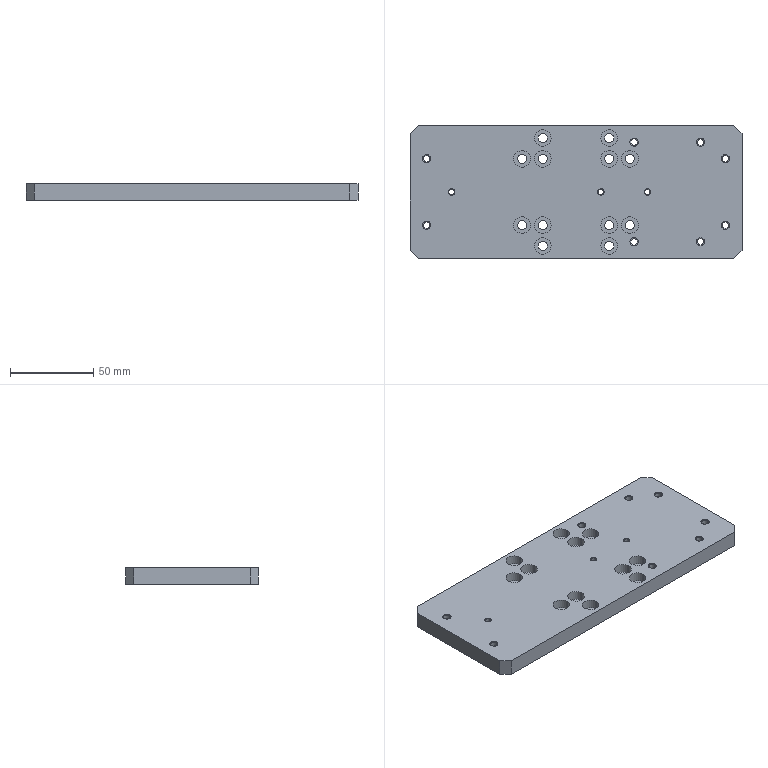Part | STEP file | 00398494_EZT_ADAPTERPLATTE_HMZV-1 | 1 solid | 120 faces | box 200 x 80 x 10 mm | volume 151646 mm3 | cylinder 70 | cone 28 | plane 22 | commonest cylinder face diameters 5.5 x24 10 x24 4.019 x16 3.141 x6